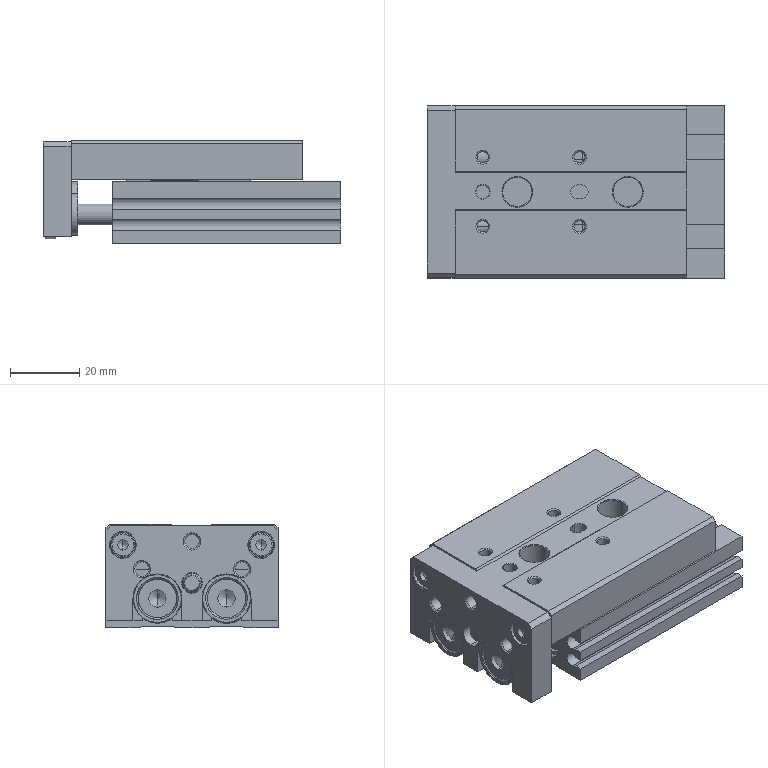Part | SolidWorks | 2 solids | 430 faces | box 86 x 50 x 30 mm | volume 87070 mm3 | plane 176 | cylinder 158 | cone 90 | spline 6 | commonest cylinder face diameters 3.242 x24 4.134 x14 12 x12 4 x10 6 x10 7.5 x8